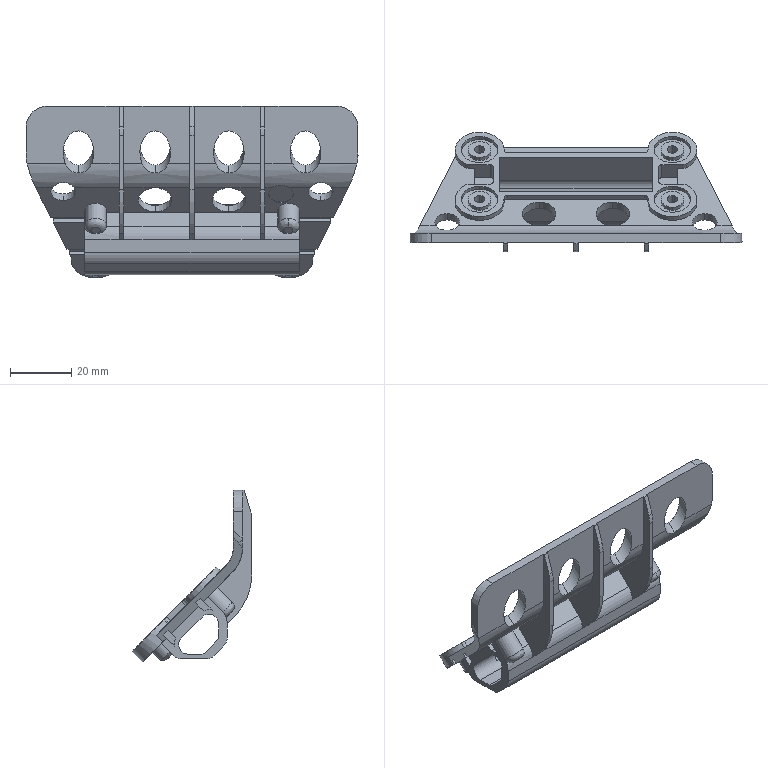Part | SolidWorks | features BaseBody 1 | 1 solid | 213 faces | box 108.193 x 39.02 x 56.008 mm | volume 23753 mm3 | plane 102 | cylinder 102 | spline 5 | cone 4 | commonest cylinder face diameters 12 x12 10 x11 2 x8 3.4 x8 7.4 x8 7 x6